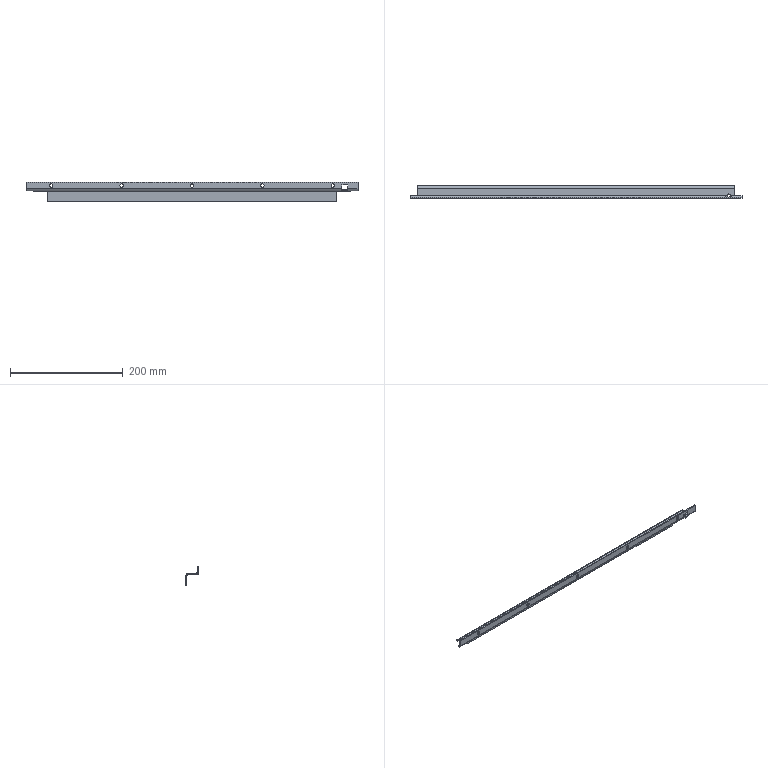Part | NX | features solid 2 | 1 solid | 44 faces | box 590 x 22 x 35 mm | volume 57677 mm3 | plane 26 | cylinder 18 | commonest cylinder face diameters 6 x12 4 x3 8 x3
STEP:
#1=CARTESIAN_POINT('',(1874.5,-1576.5,1027.));
#2=VERTEX_POINT('',#1);
#3=CARTESIAN_POINT('',(1874.5,-1576.5,1025.));
#4=VERTEX_POINT('',#3);
#5=CARTESIAN_POINT('',(1874.5,-1576.5,1616.447));
#6=DIRECTION('',(0.,0.,-1.));
#7=VECTOR('',#6,1000.);
#8=LINE('',#5,#7);
#9=EDGE_CURVE('',#2,#4,#8,.T.);
#10=ORIENTED_EDGE('',*,*,#9,.F.);
#11=CARTESIAN_POINT('',(1874.5,-1570.5,1027.));
#12=VERTEX_POINT('',#11);
#13=CARTESIAN_POINT('',(1874.5,-1573.5,1027.));
#14=DIRECTION('',(0.,0.,1.));
#15=DIRECTION('',(0.,-1.,0.));
#16=AXIS2_PLACEMENT_3D('',#13,#14,#15);
#17=CIRCLE('',#16,3.);
#18=EDGE_CURVE('',#2,#12,#17,.T.);
#19=ORIENTED_EDGE('',*,*,#18,.T.);
#20=CARTESIAN_POINT('',(1874.5,-1570.5,1025.));
#21=VERTEX_POINT('',#20);
#22=CARTESIAN_POINT('',(1874.5,-1570.5,1616.447));
#23=DIRECTION('',(0.,0.,-1.));
#24=VECTOR('',#23,1000.);
#25=LINE('',#22,#24);
#26=EDGE_CURVE('',#21,#12,#25,.F.);
#27=ORIENTED_EDGE('',*,*,#26,.F.);
#28=CARTESIAN_POINT('',(1874.5,-1573.5,1025.));
#29=DIRECTION('',(0.,0.,-1.));
#30=DIRECTION('',(1.,0.,0.));
#31=AXIS2_PLACEMENT_3D('',#28,#29,#30);
#32=CIRCLE('',#31,3.);
#33=EDGE_CURVE('',#21,#4,#32,.T.);
#34=ORIENTED_EDGE('',*,*,#33,.T.);
#35=EDGE_LOOP('',(#10,#19,#27,#34));
#36=FACE_BOUND('',#35,.T.);
#37=CARTESIAN_POINT('',(1874.5,-1573.5,1616.447));
#38=DIRECTION('',(0.,0.,-1.));
#39=DIRECTION('',(0.,1.,0.));
#40=AXIS2_PLACEMENT_3D('',#37,#38,#39);
#41=CYLINDRICAL_SURFACE('',#40,3.);
#42=ADVANCED_FACE('',(#36),#41,.F.);
#43=CARTESIAN_POINT('',(1879.4,-1574.,1025.));
#44=VERTEX_POINT('',#43);
#45=CARTESIAN_POINT('',(1879.5,-1574.,1025.));
#46=VERTEX_POINT('',#45);
#47=CARTESIAN_POINT('',(1879.5,-1574.,1025.));
#48=DIRECTION('',(1.,0.,0.));
#49=VECTOR('',#48,1000.);
#50=LINE('',#47,#49);
#51=EDGE_CURVE('',#44,#46,#50,.T.);
#52=ORIENTED_EDGE('',*,*,#51,.T.);
#53=CARTESIAN_POINT('',(1879.5,-1574.,1027.));
#54=VERTEX_POINT('',#53);
#55=CARTESIAN_POINT('',(1879.5,-1574.,1027.));
#56=DIRECTION('',(0.,0.,-1.));
#57=VECTOR('',#56,1000.);
#58=LINE('',#55,#57);
#59=EDGE_CURVE('',#54,#46,#58,.T.);
#60=ORIENTED_EDGE('',*,*,#59,.F.);
#61=CARTESIAN_POINT('',(1879.4,-1574.,1027.));
#62=VERTEX_POINT('',#61);
#63=CARTESIAN_POINT('',(1879.5,-1574.,1027.));
#64=DIRECTION('',(1.,0.,0.));
#65=VECTOR('',#64,1000.);
#66=LINE('',#63,#65);
#67=EDGE_CURVE('',#62,#54,#66,.T.);
#68=ORIENTED_EDGE('',*,*,#67,.F.);
#69=CARTESIAN_POINT('',(1879.4,-1574.,1027.));
#70=DIRECTION('',(0.,0.,-1.));
#71=VECTOR('',#70,1000.);
#72=LINE('',#69,#71);
#73=EDGE_CURVE('',#62,#44,#72,.T.);
#74=ORIENTED_EDGE('',*,*,#73,.T.);
#75=EDGE_LOOP('',(#52,#60,#68,#74));
#76=FACE_BOUND('',#75,.T.);
#77=CARTESIAN_POINT('',(1879.5,-1574.,1027.));
#78=DIRECTION('',(0.,1.,0.));
#79=DIRECTION('',(0.,0.,-1.));
#80=AXIS2_PLACEMENT_3D('',#77,#78,#79);
#81=PLANE('',#80);
#82=ADVANCED_FACE('',(#76),#81,.F.);
#83=CARTESIAN_POINT('',(1879.4,-1578.,1025.));
#84=VERTEX_POINT('',#83);
#85=CARTESIAN_POINT('',(1879.4,-1578.,1025.));
#86=DIRECTION('',(0.,1.,0.));
#87=VECTOR('',#86,1000.);
#88=LINE('',#85,#87);
#89=EDGE_CURVE('',#84,#44,#88,.T.);
#90=ORIENTED_EDGE('',*,*,#89,.T.);
#91=ORIENTED_EDGE('',*,*,#73,.F.);
#92=CARTESIAN_POINT('',(1879.4,-1578.,1027.));
#93=VERTEX_POINT('',#92);
#94=CARTESIAN_POINT('',(1879.4,-1578.,1027.));
#95=DIRECTION('',(0.,1.,0.));
#96=VECTOR('',#95,1000.);
#97=LINE('',#94,#96);
#98=EDGE_CURVE('',#93,#62,#97,.T.);
#99=ORIENTED_EDGE('',*,*,#98,.F.);
#100=CARTESIAN_POINT('',(1879.4,-1578.,1027.));
#101=DIRECTION('',(0.,0.,-1.));
#102=VECTOR('',#101,1000.);
#103=LINE('',#100,#102);
#104=EDGE_CURVE('',#93,#84,#103,.T.);
#105=ORIENTED_EDGE('',*,*,#104,.T.);
#106=EDGE_LOOP('',(#90,#91,#99,#105));
#107=FACE_BOUND('',#106,.T.);
#108=CARTESIAN_POINT('',(1879.4,-1578.,1027.));
#109=DIRECTION('',(-1.,0.,0.));
#110=DIRECTION('',(0.,0.,1.));
#111=AXIS2_PLACEMENT_3D('',#108,#109,#110);
#112=PLANE('',#111);
#113=ADVANCED_FACE('',(#107),#112,.F.);
#114=CARTESIAN_POINT('',(1869.6,-1578.,1025.));
#115=VERTEX_POINT('',#114);
#116=CARTESIAN_POINT('',(1879.4,-1578.,1025.));
#117=DIRECTION('',(1.,0.,0.));
#118=VECTOR('',#117,1000.);
#119=LINE('',#116,#118);
#120=EDGE_CURVE('',#115,#84,#119,.T.);
#121=ORIENTED_EDGE('',*,*,#120,.T.);
#122=ORIENTED_EDGE('',*,*,#104,.F.);
#123=CARTESIAN_POINT('',(1869.6,-1578.,1027.));
#124=VERTEX_POINT('',#123);
#125=CARTESIAN_POINT('',(1879.4,-1578.,1027.));
#126=DIRECTION('',(1.,0.,0.));
#127=VECTOR('',#126,1000.);
#128=LINE('',#125,#127);
#129=EDGE_CURVE('',#124,#93,#128,.T.);
#130=ORIENTED_EDGE('',*,*,#129,.F.);
#131=CARTESIAN_POINT('',(1869.6,-1578.,1027.));
#132=DIRECTION('',(0.,0.,-1.));
#133=VECTOR('',#132,1000.);
#134=LINE('',#131,#133);
#135=EDGE_CURVE('',#124,#115,#134,.T.);
#136=ORIENTED_EDGE('',*,*,#135,.T.);
#137=EDGE_LOOP('',(#121,#122,#130,#136));
#138=FACE_BOUND('',#137,.T.);
#139=CARTESIAN_POINT('',(1879.4,-1578.,1027.));
#140=DIRECTION('',(0.,1.,0.));
#141=DIRECTION('',(0.,0.,-1.));
#142=AXIS2_PLACEMENT_3D('',#139,#140,#141);
#143=PLANE('',#142);
#144=ADVANCED_FACE('',(#138),#143,.F.);
#145=CARTESIAN_POINT('',(1869.6,-1574.,1025.));
#146=VERTEX_POINT('',#145);
#147=CARTESIAN_POINT('',(1869.6,-1574.,1025.));
#148=DIRECTION('',(0.,-1.,0.));
#149=VECTOR('',#148,1000.);
#150=LINE('',#147,#149);
#151=EDGE_CURVE('',#146,#115,#150,.T.);
#152=ORIENTED_EDGE('',*,*,#151,.T.);
#153=ORIENTED_EDGE('',*,*,#135,.F.);
#154=CARTESIAN_POINT('',(1869.6,-1574.,1027.));
#155=VERTEX_POINT('',#154);
#156=CARTESIAN_POINT('',(1869.6,-1574.,1027.));
#157=DIRECTION('',(0.,-1.,0.));
#158=VECTOR('',#157,1000.);
#159=LINE('',#156,#158);
#160=EDGE_CURVE('',#155,#124,#159,.T.);
#161=ORIENTED_EDGE('',*,*,#160,.F.);
#162=CARTESIAN_POINT('',(1869.6,-1574.,1027.));
#163=DIRECTION('',(0.,0.,-1.));
#164=VECTOR('',#163,1000.);
#165=LINE('',#162,#164);
#166=EDGE_CURVE('',#155,#146,#165,.T.);
#167=ORIENTED_EDGE('',*,*,#166,.T.);
#168=EDGE_LOOP('',(#152,#153,#161,#167));
#169=FACE_BOUND('',#168,.T.);
#170=CARTESIAN_POINT('',(1869.6,-1574.,1027.));
#171=DIRECTION('',(1.,0.,0.));
#172=DIRECTION('',(0.,0.,1.));
#173=AXIS2_PLACEMENT_3D('',#170,#171,#172);
#174=PLANE('',#173);
#175=ADVANCED_FACE('',(#169),#174,.F.);
#176=CARTESIAN_POINT('',(1869.5,-1574.,1025.));
#177=VERTEX_POINT('',#176);
#178=CARTESIAN_POINT('',(1869.6,-1574.,1025.));
#179=DIRECTION('',(1.,0.,0.));
#180=VECTOR('',#179,1000.);
#181=LINE('',#178,#180);
#182=EDGE_CURVE('',#177,#146,#181,.T.);
#183=ORIENTED_EDGE('',*,*,#182,.T.);
#184=ORIENTED_EDGE('',*,*,#166,.F.);
#185=CARTESIAN_POINT('',(1869.5,-1574.,1027.));
#186=VERTEX_POINT('',#185);
#187=CARTESIAN_POINT('',(1869.6,-1574.,1027.));
#188=DIRECTION('',(1.,0.,0.));
#189=VECTOR('',#188,1000.);
#190=LINE('',#187,#189);
#191=EDGE_CURVE('',#186,#155,#190,.T.);
#192=ORIENTED_EDGE('',*,*,#191,.F.);
#193=CARTESIAN_POINT('',(1869.5,-1574.,1027.));
#194=DIRECTION('',(0.,0.,-1.));
#195=VECTOR('',#194,1000.);
#196=LINE('',#193,#195);
#197=EDGE_CURVE('',#186,#177,#196,.T.);
#198=ORIENTED_EDGE('',*,*,#197,.T.);
#199=EDGE_LOOP('',(#183,#184,#192,#198));
#200=FACE_BOUND('',#199,.T.);
#201=CARTESIAN_POINT('',(1869.6,-1574.,1027.));
#202=DIRECTION('',(0.,1.,0.));
#203=DIRECTION('',(0.,0.,-1.));
#204=AXIS2_PLACEMENT_3D('',#201,#202,#203);
#205=PLANE('',#204);
#206=ADVANCED_FACE('',(#200),#205,.F.);
#207=CARTESIAN_POINT('',(1869.5,-1576.,1035.));
#208=VERTEX_POINT('',#207);
#209=CARTESIAN_POINT('',(1869.5,-1578.,1035.));
#210=VERTEX_POINT('',#209);
#211=CARTESIAN_POINT('',(1869.5,-1578.,1035.));
#212=DIRECTION('',(0.,-1.,0.));
#213=VECTOR('',#212,1000.);
#214=LINE('',#211,#213);
#215=EDGE_CURVE('',#208,#210,#214,.T.);
#216=ORIENTED_EDGE('',*,*,#215,.F.);
#217=CARTESIAN_POINT('',(1879.5,-1576.,1035.));
#218=VERTEX_POINT('',#217);
#219=CARTESIAN_POINT('',(1898.,-1576.,1035.));
#220=DIRECTION('',(-1.,0.,0.));
#221=VECTOR('',#220,1000.);
#222=LINE('',#219,#221);
#223=EDGE_CURVE('',#218,#208,#222,.T.);
#224=ORIENTED_EDGE('',*,*,#223,.F.);
#225=CARTESIAN_POINT('',(1879.5,-1578.,1035.));
#226=VERTEX_POINT('',#225);
#227=CARTESIAN_POINT('',(1879.5,-1578.,1035.));
#228=DIRECTION('',(0.,-1.,0.));
#229=VECTOR('',#228,1000.);
#230=LINE('',#227,#229);
#231=EDGE_CURVE('',#218,#226,#230,.T.);
#232=ORIENTED_EDGE('',*,*,#231,.T.);
#233=CARTESIAN_POINT('',(1898.,-1578.,1035.));
#234=DIRECTION('',(-1.,0.,0.));
#235=VECTOR('',#234,1000.);
#236=LINE('',#233,#235);
#237=EDGE_CURVE('',#226,#210,#236,.T.);
#238=ORIENTED_EDGE('',*,*,#237,.T.);
#239=EDGE_LOOP('',(#216,#224,#232,#238));
#240=FACE_BOUND('',#239,.T.);
#241=CARTESIAN_POINT('',(1898.,-1578.,1035.));
#242=DIRECTION('',(0.,0.,-1.));
#243=DIRECTION('',(0.,-1.,0.));
#244=AXIS2_PLACEMENT_3D('',#241,#242,#243);
#245=PLANE('',#244);
#246=ADVANCED_FACE('',(#240),#245,.T.);
#247=CARTESIAN_POINT('',(1885.,-1558.,1023.));
#248=VERTEX_POINT('',#247);
#249=CARTESIAN_POINT('',(1885.,-1560.,1025.));
#250=VERTEX_POINT('',#249);
#251=CARTESIAN_POINT('',(1885.,-1560.,1023.));
#252=DIRECTION('',(1.,0.,0.));
#253=DIRECTION('',(0.,0.,-1.));
#254=AXIS2_PLACEMENT_3D('',#251,#252,#253);
#255=CIRCLE('',#254,2.);
#256=EDGE_CURVE('',#248,#250,#255,.T.);
#257=ORIENTED_EDGE('',*,*,#256,.F.);
#258=CARTESIAN_POINT('',(1885.,-1556.,1023.));
#259=VERTEX_POINT('',#258);
#260=CARTESIAN_POINT('',(1885.,-1558.,1023.));
#261=DIRECTION('',(0.,-1.,0.));
#262=VECTOR('',#261,1000.);
#263=LINE('',#260,#262);
#264=EDGE_CURVE('',#259,#248,#263,.T.);
#265=ORIENTED_EDGE('',*,*,#264,.F.);
#266=CARTESIAN_POINT('',(1885.,-1560.,1027.));
#267=VERTEX_POINT('',#266);
#268=CARTESIAN_POINT('',(1885.,-1560.,1023.));
#269=DIRECTION('',(1.,0.,0.));
#270=DIRECTION('',(0.,0.,-1.));
#271=AXIS2_PLACEMENT_3D('',#268,#269,#270);
#272=CIRCLE('',#271,4.);
#273=EDGE_CURVE('',#259,#267,#272,.T.);
#274=ORIENTED_EDGE('',*,*,#273,.T.);
#275=CARTESIAN_POINT('',(1885.,-1574.,1027.));
#276=VERTEX_POINT('',#275);
#277=CARTESIAN_POINT('',(1885.,-1578.,1027.));
#278=DIRECTION('',(0.,-1.,0.));
#279=VECTOR('',#278,1000.);
#280=LINE('',#277,#279);
#281=EDGE_CURVE('',#267,#276,#280,.T.);
#282=ORIENTED_EDGE('',*,*,#281,.T.);
#283=CARTESIAN_POINT('',(1885.,-1574.,1025.));
#284=VERTEX_POINT('',#283);
#285=CARTESIAN_POINT('',(1885.,-1574.,1025.));
#286=DIRECTION('',(0.,0.,-1.));
#287=VECTOR('',#286,1000.);
#288=LINE('',#285,#287);
#289=EDGE_CURVE('',#276,#284,#288,.T.);
#290=ORIENTED_EDGE('',*,*,#289,.T.);
#291=CARTESIAN_POINT('',(1885.,-1578.,1025.));
#292=DIRECTION('',(0.,-1.,0.));
#293=VECTOR('',#292,1000.);
#294=LINE('',#291,#293);
#295=EDGE_CURVE('',#250,#284,#294,.T.);
#296=ORIENTED_EDGE('',*,*,#295,.F.);
#297=EDGE_LOOP('',(#257,#265,#274,#282,#290,#296));
#298=FACE_BOUND('',#297,.T.);
#299=CARTESIAN_POINT('',(1885.,-1560.,1023.));
#300=DIRECTION('',(1.,0.,0.));
#301=DIRECTION('',(0.,0.,1.));
#302=AXIS2_PLACEMENT_3D('',#299,#300,#301);
#303=PLANE('',#302);
#304=ADVANCED_FACE('',(#298),#303,.T.);
#305=CARTESIAN_POINT('',(1898.,-1574.,1027.));
#306=VERTEX_POINT('',#305);
#307=CARTESIAN_POINT('',(1898.,-1574.,1025.));
#308=VERTEX_POINT('',#307);
#309=CARTESIAN_POINT('',(1898.,-1574.,1025.));
#310=DIRECTION('',(0.,0.,-1.));
#311=VECTOR('',#310,1000.);
#312=LINE('',#309,#311);
#313=EDGE_CURVE('',#306,#308,#312,.T.);
#314=ORIENTED_EDGE('',*,*,#313,.T.);
#315=CARTESIAN_POINT('',(1898.,-1574.,1025.));
#316=DIRECTION('',(-1.,0.,0.));
#317=VECTOR('',#316,1000.);
#318=LINE('',#315,#317);
#319=EDGE_CURVE('',#308,#284,#318,.T.);
#320=ORIENTED_EDGE('',*,*,#319,.T.);
#321=ORIENTED_EDGE('',*,*,#289,.F.);
#322=CARTESIAN_POINT('',(1898.,-1574.,1027.));
#323=DIRECTION('',(-1.,0.,0.));
#324=VECTOR('',#323,1000.);
#325=LINE('',#322,#324);
#326=EDGE_CURVE('',#306,#276,#325,.T.);
#327=ORIENTED_EDGE('',*,*,#326,.F.);
#328=EDGE_LOOP('',(#314,#320,#321,#327));
#329=FACE_BOUND('',#328,.T.);
#330=CARTESIAN_POINT('',(1898.,-1574.,1025.));
#331=DIRECTION('',(0.,1.,0.));
#332=DIRECTION('',(0.,0.,-1.));
#333=AXIS2_PLACEMENT_3D('',#330,#331,#332);
#334=PLANE('',#333);
#335=ADVANCED_FACE('',(#329),#334,.T.);
#336=CARTESIAN_POINT('',(1321.,-1574.,1027.));
#337=VERTEX_POINT('',#336);
#338=CARTESIAN_POINT('',(1321.,-1560.,1027.));
#339=VERTEX_POINT('',#338);
#340=CARTESIAN_POINT('',(1321.,-1578.,1027.));
#341=DIRECTION('',(0.,1.,0.));
#342=VECTOR('',#341,1000.);
#343=LINE('',#340,#342);
#344=EDGE_CURVE('',#337,#339,#343,.T.);
#345=ORIENTED_EDGE('',*,*,#344,.T.);
#346=CARTESIAN_POINT('',(1321.,-1556.,1023.));
#347=VERTEX_POINT('',#346);
#348=CARTESIAN_POINT('',(1321.,-1560.,1023.));
#349=DIRECTION('',(-1.,0.,0.));
#350=DIRECTION('',(0.,0.,-1.));
#351=AXIS2_PLACEMENT_3D('',#348,#349,#350);
#352=CIRCLE('',#351,4.);
#353=EDGE_CURVE('',#339,#347,#352,.T.);
#354=ORIENTED_EDGE('',*,*,#353,.T.);
#355=CARTESIAN_POINT('',(1321.,-1558.,1023.));
#356=VERTEX_POINT('',#355);
#357=CARTESIAN_POINT('',(1321.,-1558.,1023.));
#358=DIRECTION('',(0.,-1.,0.));
#359=VECTOR('',#358,1000.);
#360=LINE('',#357,#359);
#361=EDGE_CURVE('',#347,#356,#360,.T.);
#362=ORIENTED_EDGE('',*,*,#361,.T.);
#363=CARTESIAN_POINT('',(1321.,-1560.,1025.));
#364=VERTEX_POINT('',#363);
#365=CARTESIAN_POINT('',(1321.,-1560.,1023.));
#366=DIRECTION('',(-1.,0.,0.));
#367=DIRECTION('',(0.,0.,1.));
#368=AXIS2_PLACEMENT_3D('',#365,#366,#367);
#369=CIRCLE('',#368,2.);
#370=EDGE_CURVE('',#364,#356,#369,.T.);
#371=ORIENTED_EDGE('',*,*,#370,.F.);
#372=CARTESIAN_POINT('',(1321.,-1574.,1025.));
#373=VERTEX_POINT('',#372);
#374=CARTESIAN_POINT('',(1321.,-1578.,1025.));
#375=DIRECTION('',(0.,1.,0.));
#376=VECTOR('',#375,1000.);
#377=LINE('',#374,#376);
#378=EDGE_CURVE('',#373,#364,#377,.T.);
#379=ORIENTED_EDGE('',*,*,#378,.F.);
#380=CARTESIAN_POINT('',(1321.,-1574.,1025.));
#381=DIRECTION('',(0.,0.,-1.));
#382=VECTOR('',#381,1000.);
#383=LINE('',#380,#382);
#384=EDGE_CURVE('',#337,#373,#383,.T.);
#385=ORIENTED_EDGE('',*,*,#384,.F.);
#386=EDGE_LOOP('',(#345,#354,#362,#371,#379,#385));
#387=FACE_BOUND('',#386,.T.);
#388=CARTESIAN_POINT('',(1321.,-1578.,1025.));
#389=DIRECTION('',(1.,0.,0.));
#390=DIRECTION('',(0.,0.,1.));
#391=AXIS2_PLACEMENT_3D('',#388,#389,#390);
#392=PLANE('',#391);
#393=ADVANCED_FACE('',(#387),#392,.F.);
#394=ORIENTED_EDGE('',*,*,#384,.T.);
#395=CARTESIAN_POINT('',(1308.,-1574.,1025.));
#396=VERTEX_POINT('',#395);
#397=CARTESIAN_POINT('',(1898.,-1574.,1025.));
#398=DIRECTION('',(-1.,0.,0.));
#399=VECTOR('',#398,1000.);
#400=LINE('',#397,#399);
#401=EDGE_CURVE('',#373,#396,#400,.T.);
#402=ORIENTED_EDGE('',*,*,#401,.T.);
#403=CARTESIAN_POINT('',(1308.,-1574.,1027.));
#404=VERTEX_POINT('',#403);
#405=CARTESIAN_POINT('',(1308.,-1574.,1025.));
#406=DIRECTION('',(0.,0.,-1.));
#407=VECTOR('',#406,1000.);
#408=LINE('',#405,#407);
#409=EDGE_CURVE('',#404,#396,#408,.T.);
#410=ORIENTED_EDGE('',*,*,#409,.F.);
#411=CARTESIAN_POINT('',(1898.,-1574.,1027.));
#412=DIRECTION('',(-1.,0.,0.));
#413=VECTOR('',#412,1000.);
#414=LINE('',#411,#413);
#415=EDGE_CURVE('',#337,#404,#414,.T.);
#416=ORIENTED_EDGE('',*,*,#415,.F.);
#417=EDGE_LOOP('',(#394,#402,#410,#416));
#418=FACE_BOUND('',#417,.T.);
#419=CARTESIAN_POINT('',(1898.,-1574.,1025.));
#420=DIRECTION('',(0.,1.,0.));
#421=DIRECTION('',(0.,0.,-1.));
#422=AXIS2_PLACEMENT_3D('',#419,#420,#421);
#423=PLANE('',#422);
#424=ADVANCED_FACE('',(#418),#423,.T.);
#425=CARTESIAN_POINT('',(1603.,-1578.,1031.));
#426=VERTEX_POINT('',#425);
#427=CARTESIAN_POINT('',(1603.,-1576.,1031.));
#428=VERTEX_POINT('',#427);
#429=CARTESIAN_POINT('',(1603.,-2167.447,1031.));
#430=DIRECTION('',(0.,1.,0.));
#431=VECTOR('',#430,1000.);
#432=LINE('',#429,#431);
#433=EDGE_CURVE('',#426,#428,#432,.T.);
#434=ORIENTED_EDGE('',*,*,#433,.F.);
#435=CARTESIAN_POINT('',(1603.,-1578.,1037.));
#436=VERTEX_POINT('',#435);
#437=CARTESIAN_POINT('',(1603.,-1578.,1034.));
#438=DIRECTION('',(0.,1.,0.));
#439=DIRECTION('',(0.,0.,1.));
#440=AXIS2_PLACEMENT_3D('',#437,#438,#439);
#441=CIRCLE('',#440,3.);
#442=EDGE_CURVE('',#436,#426,#441,.T.);
#443=ORIENTED_EDGE('',*,*,#442,.F.);
#444=CARTESIAN_POINT('',(1603.,-1576.,1037.));
#445=VERTEX_POINT('',#444);
#446=CARTESIAN_POINT('',(1603.,-2167.447,1037.));
#447=DIRECTION('',(0.,1.,0.));
#448=VECTOR('',#447,1000.);
#449=LINE('',#446,#448);
#450=EDGE_CURVE('',#445,#436,#449,.F.);
#451=ORIENTED_EDGE('',*,*,#450,.F.);
#452=CARTESIAN_POINT('',(1603.,-1576.,1034.));
#453=DIRECTION('',(0.,1.,0.));
#454=DIRECTION('',(-1.,0.,0.));
#455=AXIS2_PLACEMENT_3D('',#452,#453,#454);
#456=CIRCLE('',#455,3.);
#457=EDGE_CURVE('',#445,#428,#456,.T.);
#458=ORIENTED_EDGE('',*,*,#457,.T.);
#459=EDGE_LOOP('',(#434,#443,#451,#458));
#460=FACE_BOUND('',#459,.T.);
#461=CARTESIAN_POINT('',(1603.,-2167.447,1034.));
#462=DIRECTION('',(0.,1.,0.));
#463=DIRECTION('',(0.,0.,1.));
#464=AXIS2_PLACEMENT_3D('',#461,#462,#463);
#465=CYLINDRICAL_SURFACE('',#464,3.);
#466=ADVANCED_FACE('',(#460),#465,.F.);
#467=CARTESIAN_POINT('',(1853.,-1578.,1031.));
#468=VERTEX_POINT('',#467);
#469=CARTESIAN_POINT('',(1853.,-1576.,1031.));
#470=VERTEX_POINT('',#469);
#471=CARTESIAN_POINT('',(1853.,-2167.447,1031.));
#472=DIRECTION('',(0.,1.,0.));
#473=VECTOR('',#472,1000.);
#474=LINE('',#471,#473);
#475=EDGE_CURVE('',#468,#470,#474,.T.);
#476=ORIENTED_EDGE('',*,*,#475,.F.);
#477=CARTESIAN_POINT('',(1853.,-1578.,1037.));
#478=VERTEX_POINT('',#477);
#479=CARTESIAN_POINT('',(1853.,-1578.,1034.));
#480=DIRECTION('',(0.,1.,0.));
#481=DIRECTION('',(0.,0.,1.));
#482=AXIS2_PLACEMENT_3D('',#479,#480,#481);
#483=CIRCLE('',#482,3.);
#484=EDGE_CURVE('',#478,#468,#483,.T.);
#485=ORIENTED_EDGE('',*,*,#484,.F.);
#486=CARTESIAN_POINT('',(1853.,-1576.,1037.));
#487=VERTEX_POINT('',#486);
#488=CARTESIAN_POINT('',(1853.,-2167.447,1037.));
#489=DIRECTION('',(0.,1.,0.));
#490=VECTOR('',#489,1000.);
#491=LINE('',#488,#490);
#492=EDGE_CURVE('',#487,#478,#491,.F.);
#493=ORIENTED_EDGE('',*,*,#492,.F.);
#494=CARTESIAN_POINT('',(1853.,-1576.,1034.));
#495=DIRECTION('',(0.,1.,0.));
#496=DIRECTION('',(-1.,0.,0.));
#497=AXIS2_PLACEMENT_3D('',#494,#495,#496);
#498=CIRCLE('',#497,3.);
#499=EDGE_CURVE('',#487,#470,#498,.T.);
#500=ORIENTED_EDGE('',*,*,#499,.T.);
#501=EDGE_LOOP('',(#476,#485,#493,#500));
#502=FACE_BOUND('',#501,.T.);
#503=CARTESIAN_POINT('',(1853.,-2167.447,1034.));
#504=DIRECTION('',(0.,1.,0.));
#505=DIRECTION('',(0.,0.,1.));
#506=AXIS2_PLACEMENT_3D('',#503,#504,#505);
#507=CYLINDRICAL_SURFACE('',#506,3.);
#508=ADVANCED_FACE('',(#502),#507,.F.);
#509=CARTESIAN_POINT('',(1728.,-1578.,1031.));
#510=VERTEX_POINT('',#509);
#511=CARTESIAN_POINT('',(1728.,-1576.,1031.));
#512=VERTEX_POINT('',#511);
#513=CARTESIAN_POINT('',(1728.,-2167.447,1031.));
#514=DIRECTION('',(0.,1.,0.));
#515=VECTOR('',#514,1000.);
#516=LINE('',#513,#515);
#517=EDGE_CURVE('',#510,#512,#516,.T.);
#518=ORIENTED_EDGE('',*,*,#517,.F.);
#519=CARTESIAN_POINT('',(1728.,-1578.,1037.));
#520=VERTEX_POINT('',#519);
#521=CARTESIAN_POINT('',(1728.,-1578.,1034.));
#522=DIRECTION('',(0.,1.,0.));
#523=DIRECTION('',(0.,0.,1.));
#524=AXIS2_PLACEMENT_3D('',#521,#522,#523);
#525=CIRCLE('',#524,3.);
#526=EDGE_CURVE('',#520,#510,#525,.T.);
#527=ORIENTED_EDGE('',*,*,#526,.F.);
#528=CARTESIAN_POINT('',(1728.,-1576.,1037.));
#529=VERTEX_POINT('',#528);
#530=CARTESIAN_POINT('',(1728.,-2167.447,1037.));
#531=DIRECTION('',(0.,1.,0.));
#532=VECTOR('',#531,1000.);
#533=LINE('',#530,#532);
#534=EDGE_CURVE('',#529,#520,#533,.F.);
#535=ORIENTED_EDGE('',*,*,#534,.F.);
#536=CARTESIAN_POINT('',(1728.,-1576.,1034.));
#537=DIRECTION('',(0.,1.,0.));
#538=DIRECTION('',(-1.,0.,0.));
#539=AXIS2_PLACEMENT_3D('',#536,#537,#538);
#540=CIRCLE('',#539,3.);
#541=EDGE_CURVE('',#529,#512,#540,.T.);
#542=ORIENTED_EDGE('',*,*,#541,.T.);
#543=EDGE_LOOP('',(#518,#527,#535,#542));
#544=FACE_BOUND('',#543,.T.);
#545=CARTESIAN_POINT('',(1728.,-2167.447,1034.));
#546=DIRECTION('',(0.,1.,0.));
#547=DIRECTION('',(0.,0.,1.));
#548=AXIS2_PLACEMENT_3D('',#545,#546,#547);
#549=CYLINDRICAL_SURFACE('',#548,3.);
#550=ADVANCED_FACE('',(#544),#549,.F.);
#551=CARTESIAN_POINT('',(1353.,-1578.,1031.));
#552=VERTEX_POINT('',#551);
#553=CARTESIAN_POINT('',(1353.,-1576.,1031.));
#554=VERTEX_POINT('',#553);
#555=CARTESIAN_POINT('',(1353.,-2167.447,1031.));
#556=DIRECTION('',(0.,1.,0.));
#557=VECTOR('',#556,1000.);
#558=LINE('',#555,#557);
#559=EDGE_CURVE('',#552,#554,#558,.T.);
#560=ORIENTED_EDGE('',*,*,#559,.F.);
#561=CARTESIAN_POINT('',(1353.,-1578.,1037.));
#562=VERTEX_POINT('',#561);
#563=CARTESIAN_POINT('',(1353.,-1578.,1034.));
#564=DIRECTION('',(0.,1.,0.));
#565=DIRECTION('',(0.,0.,1.));
#566=AXIS2_PLACEMENT_3D('',#563,#564,#565);
#567=CIRCLE('',#566,3.);
#568=EDGE_CURVE('',#562,#552,#567,.T.);
#569=ORIENTED_EDGE('',*,*,#568,.F.);
#570=CARTESIAN_POINT('',(1353.,-1576.,1037.));
#571=VERTEX_POINT('',#570);
#572=CARTESIAN_POINT('',(1353.,-2167.447,1037.));
#573=DIRECTION('',(0.,1.,0.));
#574=VECTOR('',#573,1000.);
#575=LINE('',#572,#574);
#576=EDGE_CURVE('',#571,#562,#575,.F.);
#577=ORIENTED_EDGE('',*,*,#576,.F.);
#578=CARTESIAN_POINT('',(1353.,-1576.,1034.));
#579=DIRECTION('',(0.,1.,0.));
#580=DIRECTION('',(-1.,0.,0.));
#581=AXIS2_PLACEMENT_3D('',#578,#579,#580);
#582=CIRCLE('',#581,3.);
#583=EDGE_CURVE('',#571,#554,#582,.T.);
#584=ORIENTED_EDGE('',*,*,#583,.T.);
#585=EDGE_LOOP('',(#560,#569,#577,#584));
#586=FACE_BOUND('',#585,.T.);
#587=CARTESIAN_POINT('',(1353.,-2167.447,1034.));
#588=DIRECTION('',(0.,1.,0.));
#589=DIRECTION('',(0.,0.,1.));
#590=AXIS2_PLACEMENT_3D('',#587,#588,#589);
#591=CYLINDRICAL_SURFACE('',#590,3.);
#592=ADVANCED_FACE('',(#586),#591,.F.);
#593=CARTESIAN_POINT('',(1478.,-1578.,1031.));
#594=VERTEX_POINT('',#593);
#595=CARTESIAN_POINT('',(1478.,-1576.,1031.));
#596=VERTEX_POINT('',#595);
#597=CARTESIAN_POINT('',(1478.,-2167.447,1031.));
#598=DIRECTION('',(0.,1.,0.));
#599=VECTOR('',#598,1000.);
#600=LINE('',#597,#599);
#601=EDGE_CURVE('',#594,#596,#600,.T.);
#602=ORIENTED_EDGE('',*,*,#601,.F.);
#603=CARTESIAN_POINT('',(1478.,-1578.,1037.));
#604=VERTEX_POINT('',#603);
#605=CARTESIAN_POINT('',(1478.,-1578.,1034.));
#606=DIRECTION('',(0.,1.,0.));
#607=DIRECTION('',(0.,0.,1.));
#608=AXIS2_PLACEMENT_3D('',#605,#606,#607);
#609=CIRCLE('',#608,3.);
#610=EDGE_CURVE('',#604,#594,#609,.T.);
#611=ORIENTED_EDGE('',*,*,#610,.F.);
#612=CARTESIAN_POINT('',(1478.,-1576.,1037.));
#613=VERTEX_POINT('',#612);
#614=CARTESIAN_POINT('',(1478.,-2167.447,1037.));
#615=DIRECTION('',(0.,1.,0.));
#616=VECTOR('',#615,1000.);
#617=LINE('',#614,#616);
#618=EDGE_CURVE('',#613,#604,#617,.F.);
#619=ORIENTED_EDGE('',*,*,#618,.F.);
#620=CARTESIAN_POINT('',(1478.,-1576.,1034.));
#621=DIRECTION('',(0.,1.,0.));
#622=DIRECTION('',(-1.,0.,0.));
#623=AXIS2_PLACEMENT_3D('',#620,#621,#622);
#624=CIRCLE('',#623,3.);
#625=EDGE_CURVE('',#613,#596,#624,.T.);
#626=ORIENTED_EDGE('',*,*,#625,.T.);
#627=EDGE_LOOP('',(#602,#611,#619,#626));
#628=FACE_BOUND('',#627,.T.);
#629=CARTESIAN_POINT('',(1478.,-2167.447,1034.));
#630=DIRECTION('',(0.,1.,0.));
#631=DIRECTION('',(0.,0.,1.));
#632=AXIS2_PLACEMENT_3D('',#629,#630,#631);
#633=CYLINDRICAL_SURFACE('',#632,3.);
#634=ADVANCED_FACE('',(#628),#633,.F.);
#635=CARTESIAN_POINT('',(1860.,-1556.,1023.));
#636=VERTEX_POINT('',#635);
#637=CARTESIAN_POINT('',(1860.,-1558.,1023.));
#638=VERTEX_POINT('',#637);
#639=CARTESIAN_POINT('',(1860.,-1558.,1023.));
#640=DIRECTION('',(0.,-1.,0.));
#641=VECTOR('',#640,1000.);
#642=LINE('',#639,#641);
#643=EDGE_CURVE('',#636,#638,#642,.T.);
#644=ORIENTED_EDGE('',*,*,#643,.T.);
#645=CARTESIAN_POINT('',(1860.,-1558.,1005.));
#646=VERTEX_POINT('',#645);
#647=CARTESIAN_POINT('',(1860.,-1558.,1025.));
#648=DIRECTION('',(0.,0.,1.));
#649=VECTOR('',#648,1000.);
#650=LINE('',#647,#649);
#651=EDGE_CURVE('',#646,#638,#650,.T.);
#652=ORIENTED_EDGE('',*,*,#651,.F.);
#653=CARTESIAN_POINT('',(1860.,-1556.,1005.));
#654=VERTEX_POINT('',#653);
#655=CARTESIAN_POINT('',(1860.,-1558.,1005.));
#656=DIRECTION('',(0.,-1.,0.));
#657=VECTOR('',#656,1000.);
#658=LINE('',#655,#657);
#659=EDGE_CURVE('',#654,#646,#658,.T.);
#660=ORIENTED_EDGE('',*,*,#659,.F.);
#661=CARTESIAN_POINT('',(1860.,-1556.,1025.));
#662=DIRECTION('',(0.,0.,1.));
#663=VECTOR('',#662,1000.);
#664=LINE('',#661,#663);
#665=EDGE_CURVE('',#654,#636,#664,.T.);
#666=ORIENTED_EDGE('',*,*,#665,.T.);
#667=EDGE_LOOP('',(#644,#652,#660,#666));
#668=FACE_BOUND('',#667,.T.);
#669=CARTESIAN_POINT('',(1860.,-1558.,1025.));
#670=DIRECTION('',(-1.,0.,0.));
#671=DIRECTION('',(0.,0.,1.));
#672=AXIS2_PLACEMENT_3D('',#669,#670,#671);
#673=PLANE('',#672);
#674=ADVANCED_FACE('',(#668),#673,.F.);
#675=CARTESIAN_POINT('',(1898.,-1556.,1023.));
#676=DIRECTION('',(-1.,0.,0.));
#677=VECTOR('',#676,1000.);
#678=LINE('',#675,#677);
#679=EDGE_CURVE('',#259,#636,#678,.T.);
#680=ORIENTED_EDGE('',*,*,#679,.F.);
#681=ORIENTED_EDGE('',*,*,#264,.T.);
#682=CARTESIAN_POINT('',(1898.,-1558.,1023.));
#683=DIRECTION('',(-1.,0.,0.));
#684=VECTOR('',#683,1000.);
#685=LINE('',#682,#684);
#686=EDGE_CURVE('',#248,#638,#685,.T.);
#687=ORIENTED_EDGE('',*,*,#686,.T.);
#688=ORIENTED_EDGE('',*,*,#643,.F.);
#689=EDGE_LOOP('',(#680,#681,#687,#688));
#690=FACE_BOUND('',#689,.T.);
#691=CARTESIAN_POINT('',(1898.,-1558.,1023.));
#692=DIRECTION('',(0.,0.,-1.));
#693=DIRECTION('',(0.,-1.,0.));
#694=AXIS2_PLACEMENT_3D('',#691,#692,#693);
#695=PLANE('',#694);
#696=ADVANCED_FACE('',(#690),#695,.T.);
#697=CARTESIAN_POINT('',(1346.,-1556.,1005.));
#698=VERTEX_POINT('',#697);
#699=CARTESIAN_POINT('',(1346.,-1556.,1023.));
#700=VERTEX_POINT('',#699);
#701=CARTESIAN_POINT('',(1346.,-1556.,1025.));
#702=DIRECTION('',(0.,0.,1.));
#703=VECTOR('',#702,1000.);
#704=LINE('',#701,#703);
#705=EDGE_CURVE('',#698,#700,#704,.T.);
#706=ORIENTED_EDGE('',*,*,#705,.F.);
#707=CARTESIAN_POINT('',(1346.,-1558.,1005.));
#708=VERTEX_POINT('',#707);
#709=CARTESIAN_POINT('',(1346.,-1558.,1005.));
#710=DIRECTION('',(0.,-1.,0.));
#711=VECTOR('',#710,1000.);
#712=LINE('',#709,#711);
#713=EDGE_CURVE('',#698,#708,#712,.T.);
#714=ORIENTED_EDGE('',*,*,#713,.T.);
#715=CARTESIAN_POINT('',(1346.,-1558.,1023.));
#716=VERTEX_POINT('',#715);
#717=CARTESIAN_POINT('',(1346.,-1558.,1025.));
#718=DIRECTION('',(0.,0.,1.));
#719=VECTOR('',#718,1000.);
#720=LINE('',#717,#719);
#721=EDGE_CURVE('',#708,#716,#720,.T.);
#722=ORIENTED_EDGE('',*,*,#721,.T.);
#723=CARTESIAN_POINT('',(1346.,-1558.,1023.));
#724=DIRECTION('',(0.,-1.,0.));
#725=VECTOR('',#724,1000.);
#726=LINE('',#723,#725);
#727=EDGE_CURVE('',#700,#716,#726,.T.);
#728=ORIENTED_EDGE('',*,*,#727,.F.);
#729=EDGE_LOOP('',(#706,#714,#722,#728));
#730=FACE_BOUND('',#729,.T.);
#731=CARTESIAN_POINT('',(1346.,-1558.,1025.));
#732=DIRECTION('',(-1.,0.,0.));
#733=DIRECTION('',(0.,0.,1.));
#734=AXIS2_PLACEMENT_3D('',#731,#732,#733);
#735=PLANE('',#734);
#736=ADVANCED_FACE('',(#730),#735,.T.);
#737=CARTESIAN_POINT('',(1898.,-1558.,1005.));
#738=DIRECTION('',(-1.,0.,0.));
#739=VECTOR('',#738,1000.);
#740=LINE('',#737,#739);
#741=EDGE_CURVE('',#646,#708,#740,.T.);
#742=ORIENTED_EDGE('',*,*,#741,.F.);
#743=ORIENTED_EDGE('',*,*,#651,.T.);
#744=CARTESIAN_POINT('',(1898.,-1558.,1023.));
#745=DIRECTION('',(-1.,0.,0.));
#746=VECTOR('',#745,1000.);
#747=LINE('',#744,#746);
#748=EDGE_CURVE('',#638,#716,#747,.T.);
#749=ORIENTED_EDGE('',*,*,#748,.T.);
#750=ORIENTED_EDGE('',*,*,#721,.F.);
#751=EDGE_LOOP('',(#742,#743,#749,#750));
#752=FACE_BOUND('',#751,.T.);
#753=CARTESIAN_POINT('',(1898.,-1558.,1025.));
#754=DIRECTION('',(0.,1.,0.));
#755=DIRECTION('',(0.,0.,-1.));
#756=AXIS2_PLACEMENT_3D('',#753,#754,#755);
#757=PLANE('',#756);
#758=ADVANCED_FACE('',(#752),#757,.F.);
#759=ORIENTED_EDGE('',*,*,#686,.F.);
#760=ORIENTED_EDGE('',*,*,#256,.T.);
#761=CARTESIAN_POINT('',(1898.,-1560.,1025.));
#762=DIRECTION('',(-1.,0.,0.));
#763=VECTOR('',#762,1000.);
#764=LINE('',#761,#763);
#765=EDGE_CURVE('',#250,#364,#764,.T.);
#766=ORIENTED_EDGE('',*,*,#765,.T.);
#767=ORIENTED_EDGE('',*,*,#370,.T.);
#768=CARTESIAN_POINT('',(1898.,-1558.,1023.));
#769=DIRECTION('',(-1.,0.,0.));
#770=VECTOR('',#769,1000.);
#771=LINE('',#768,#770);
#772=EDGE_CURVE('',#716,#356,#771,.T.);
#773=ORIENTED_EDGE('',*,*,#772,.F.);
#774=ORIENTED_EDGE('',*,*,#748,.F.);
#775=EDGE_LOOP('',(#759,#760,#766,#767,#773,#774));
#776=FACE_BOUND('',#775,.T.);
#777=CARTESIAN_POINT('',(1898.,-1560.,1023.));
#778=DIRECTION('',(-1.,0.,0.));
#779=DIRECTION('',(0.,0.,-1.));
#780=AXIS2_PLACEMENT_3D('',#777,#778,#779);
#781=CYLINDRICAL_SURFACE('',#780,2.);
#782=ADVANCED_FACE('',(#776),#781,.F.);
#783=ORIENTED_EDGE('',*,*,#33,.F.);
#784=CARTESIAN_POINT('',(1874.5,-1573.5,1025.));
#785=DIRECTION('',(0.,0.,-1.));
#786=DIRECTION('',(1.,0.,0.));
#787=AXIS2_PLACEMENT_3D('',#784,#785,#786);
#788=CIRCLE('',#787,3.);
#789=EDGE_CURVE('',#4,#21,#788,.T.);
#790=ORIENTED_EDGE('',*,*,#789,.F.);
#791=EDGE_LOOP('',(#783,#790));
#792=FACE_BOUND('',#791,.T.);
#793=ORIENTED_EDGE('',*,*,#182,.F.);
#794=CARTESIAN_POINT('',(1898.,-1574.,1025.));
#795=DIRECTION('',(-1.,0.,0.));
#796=VECTOR('',#795,1000.);
#797=LINE('',#794,#796);
#798=EDGE_CURVE('',#177,#373,#797,.T.);
#799=ORIENTED_EDGE('',*,*,#798,.T.);
#800=ORIENTED_EDGE('',*,*,#378,.T.);
#801=ORIENTED_EDGE('',*,*,#765,.F.);
#802=ORIENTED_EDGE('',*,*,#295,.T.);
#803=CARTESIAN_POINT('',(1898.,-1574.,1025.));
#804=DIRECTION('',(-1.,0.,0.));
#805=VECTOR('',#804,1000.);
#806=LINE('',#803,#805);
#807=EDGE_CURVE('',#284,#46,#806,.T.);
#808=ORIENTED_EDGE('',*,*,#807,.T.);
#809=ORIENTED_EDGE('',*,*,#51,.F.);
#810=ORIENTED_EDGE('',*,*,#89,.F.);
#811=ORIENTED_EDGE('',*,*,#120,.F.);
#812=ORIENTED_EDGE('',*,*,#151,.F.);
#813=EDGE_LOOP('',(#793,#799,#800,#801,#802,#808,#809,#810,#811,#812));
#814=FACE_BOUND('',#813,.T.);
#815=CARTESIAN_POINT('',(1898.,-1578.,1025.));
#816=DIRECTION('',(0.,0.,1.));
#817=DIRECTION('',(1.,0.,0.));
#818=AXIS2_PLACEMENT_3D('',#815,#816,#817);
#819=PLANE('',#818);
#820=ADVANCED_FACE('',(#792,#814),#819,.F.);
#821=ORIENTED_EDGE('',*,*,#798,.F.);
#822=CARTESIAN_POINT('',(1869.5,-1578.,1029.));
#823=VERTEX_POINT('',#822);
#824=CARTESIAN_POINT('',(1869.5,-1574.,1029.));
#825=DIRECTION('',(-1.,0.,0.));
#826=DIRECTION('',(0.,0.,-1.));
#827=AXIS2_PLACEMENT_3D('',#824,#825,#826);
#828=CIRCLE('',#827,4.);
#829=EDGE_CURVE('',#177,#823,#828,.T.);
#830=ORIENTED_EDGE('',*,*,#829,.T.);
#831=CARTESIAN_POINT('',(1308.,-1578.,1029.));
#832=VERTEX_POINT('',#831);
#833=CARTESIAN_POINT('',(1898.,-1578.,1029.));
#834=DIRECTION('',(-1.,0.,0.));
#835=VECTOR('',#834,1000.);
#836=LINE('',#833,#835);
#837=EDGE_CURVE('',#823,#832,#836,.T.);
#838=ORIENTED_EDGE('',*,*,#837,.T.);
#839=CARTESIAN_POINT('',(1308.,-1574.,1029.));
#840=DIRECTION('',(1.,0.,0.));
#841=DIRECTION('',(0.,0.,-1.));
#842=AXIS2_PLACEMENT_3D('',#839,#840,#841);
#843=CIRCLE('',#842,4.);
#844=EDGE_CURVE('',#832,#396,#843,.T.);
#845=ORIENTED_EDGE('',*,*,#844,.T.);
#846=ORIENTED_EDGE('',*,*,#401,.F.);
#847=EDGE_LOOP('',(#821,#830,#838,#845,#846));
#848=FACE_BOUND('',#847,.T.);
#849=CARTESIAN_POINT('',(1898.,-1574.,1029.));
#850=DIRECTION('',(-1.,0.,0.));
#851=DIRECTION('',(0.,0.,-1.));
#852=AXIS2_PLACEMENT_3D('',#849,#850,#851);
#853=CYLINDRICAL_SURFACE('',#852,4.);
#854=ADVANCED_FACE('',(#848),#853,.T.);
#855=ORIENTED_EDGE('',*,*,#610,.T.);
#856=CARTESIAN_POINT('',(1478.,-1578.,1034.));
#857=DIRECTION('',(0.,1.,0.));
#858=DIRECTION('',(0.,0.,1.));
#859=AXIS2_PLACEMENT_3D('',#856,#857,#858);
#860=CIRCLE('',#859,3.);
#861=EDGE_CURVE('',#594,#604,#860,.T.);
#862=ORIENTED_EDGE('',*,*,#861,.T.);
#863=EDGE_LOOP('',(#855,#862));
#864=FACE_BOUND('',#863,.T.);
#865=ORIENTED_EDGE('',*,*,#568,.T.);
#866=CARTESIAN_POINT('',(1353.,-1578.,1034.));
#867=DIRECTION('',(0.,1.,0.));
#868=DIRECTION('',(0.,0.,1.));
#869=AXIS2_PLACEMENT_3D('',#866,#867,#868);
#870=CIRCLE('',#869,3.);
#871=EDGE_CURVE('',#552,#562,#870,.T.);
#872=ORIENTED_EDGE('',*,*,#871,.T.);
#873=EDGE_LOOP('',(#865,#872));
#874=FACE_BOUND('',#873,.T.);
#875=ORIENTED_EDGE('',*,*,#526,.T.);
#876=CARTESIAN_POINT('',(1728.,-1578.,1034.));
#877=DIRECTION('',(0.,1.,0.));
#878=DIRECTION('',(0.,0.,1.));
#879=AXIS2_PLACEMENT_3D('',#876,#877,#878);
#880=CIRCLE('',#879,3.);
#881=EDGE_CURVE('',#510,#520,#880,.T.);
#882=ORIENTED_EDGE('',*,*,#881,.T.);
#883=EDGE_LOOP('',(#875,#882));
#884=FACE_BOUND('',#883,.T.);
#885=ORIENTED_EDGE('',*,*,#484,.T.);
#886=CARTESIAN_POINT('',(1853.,-1578.,1034.));
#887=DIRECTION('',(0.,1.,0.));
#888=DIRECTION('',(0.,0.,1.));
#889=AXIS2_PLACEMENT_3D('',#886,#887,#888);
#890=CIRCLE('',#889,3.);
#891=EDGE_CURVE('',#468,#478,#890,.T.);
#892=ORIENTED_EDGE('',*,*,#891,.T.);
#893=EDGE_LOOP('',(#885,#892));
#894=FACE_BOUND('',#893,.T.);
#895=ORIENTED_EDGE('',*,*,#442,.T.);
#896=CARTESIAN_POINT('',(1603.,-1578.,1034.));
#897=DIRECTION('',(0.,1.,0.));
#898=DIRECTION('',(0.,0.,1.));
#899=AXIS2_PLACEMENT_3D('',#896,#897,#898);
#900=CIRCLE('',#899,3.);
#901=EDGE_CURVE('',#426,#436,#900,.T.);
#902=ORIENTED_EDGE('',*,*,#901,.T.);
#903=EDGE_LOOP('',(#895,#902));
#904=FACE_BOUND('',#903,.T.);
#905=ORIENTED_EDGE('',*,*,#237,.F.);
#906=CARTESIAN_POINT('',(1879.5,-1578.,1029.));
#907=VERTEX_POINT('',#906);
#908=CARTESIAN_POINT('',(1879.5,-1578.,1040.));
#909=DIRECTION('',(0.,0.,-1.));
#910=VECTOR('',#909,1000.);
#911=LINE('',#908,#910);
#912=EDGE_CURVE('',#226,#907,#911,.T.);
#913=ORIENTED_EDGE('',*,*,#912,.T.);
#914=CARTESIAN_POINT('',(1898.,-1578.,1029.));
#915=VERTEX_POINT('',#914);
#916=CARTESIAN_POINT('',(1898.,-1578.,1029.));
#917=DIRECTION('',(-1.,0.,0.));
#918=VECTOR('',#917,1000.);
#919=LINE('',#916,#918);
#920=EDGE_CURVE('',#915,#907,#919,.T.);
#921=ORIENTED_EDGE('',*,*,#920,.F.);
#922=CARTESIAN_POINT('',(1898.,-1578.,1040.));
#923=VERTEX_POINT('',#922);
#924=CARTESIAN_POINT('',(1898.,-1578.,1040.));
#925=DIRECTION('',(0.,0.,-1.));
#926=VECTOR('',#925,1000.);
#927=LINE('',#924,#926);
#928=EDGE_CURVE('',#923,#915,#927,.T.);
#929=ORIENTED_EDGE('',*,*,#928,.F.);
#930=CARTESIAN_POINT('',(1308.,-1578.,1040.));
#931=VERTEX_POINT('',#930);
#932=CARTESIAN_POINT('',(1898.,-1578.,1040.));
#933=DIRECTION('',(-1.,0.,0.));
#934=VECTOR('',#933,1000.);
#935=LINE('',#932,#934);
#936=EDGE_CURVE('',#923,#931,#935,.T.);
#937=ORIENTED_EDGE('',*,*,#936,.T.);
#938=CARTESIAN_POINT('',(1308.,-1578.,1040.));
#939=DIRECTION('',(0.,0.,-1.));
#940=VECTOR('',#939,1000.);
#941=LINE('',#938,#940);
#942=EDGE_CURVE('',#931,#832,#941,.T.);
#943=ORIENTED_EDGE('',*,*,#942,.T.);
#944=ORIENTED_EDGE('',*,*,#837,.F.);
#945=CARTESIAN_POINT('',(1869.5,-1578.,1040.));
#946=DIRECTION('',(0.,0.,1.));
#947=VECTOR('',#946,1000.);
#948=LINE('',#945,#947);
#949=EDGE_CURVE('',#823,#210,#948,.T.);
#950=ORIENTED_EDGE('',*,*,#949,.T.);
#951=EDGE_LOOP('',(#905,#913,#921,#929,#937,#943,#944,#950));
#952=FACE_BOUND('',#951,.T.);
#953=CARTESIAN_POINT('',(1898.,-1578.,1040.));
#954=DIRECTION('',(0.,1.,0.));
#955=DIRECTION('',(0.,0.,-1.));
#956=AXIS2_PLACEMENT_3D('',#953,#954,#955);
#957=PLANE('',#956);
#958=ADVANCED_FACE('',(#864,#874,#884,#894,#904,#952),#957,.F.);
#959=ORIENTED_EDGE('',*,*,#665,.F.);
#960=CARTESIAN_POINT('',(1898.,-1556.,1005.));
#961=DIRECTION('',(-1.,0.,0.));
#962=VECTOR('',#961,1000.);
#963=LINE('',#960,#962);
#964=EDGE_CURVE('',#654,#698,#963,.T.);
#965=ORIENTED_EDGE('',*,*,#964,.T.);
#966=ORIENTED_EDGE('',*,*,#705,.T.);
#967=CARTESIAN_POINT('',(1898.,-1556.,1023.));
#968=DIRECTION('',(-1.,0.,0.));
#969=VECTOR('',#968,1000.);
#970=LINE('',#967,#969);
#971=EDGE_CURVE('',#636,#700,#970,.T.);
#972=ORIENTED_EDGE('',*,*,#971,.F.);
#973=EDGE_LOOP('',(#959,#965,#966,#972));
#974=FACE_BOUND('',#973,.T.);
#975=CARTESIAN_POINT('',(1898.,-1556.,1025.));
#976=DIRECTION('',(0.,1.,0.));
#977=DIRECTION('',(0.,0.,-1.));
#978=AXIS2_PLACEMENT_3D('',#975,#976,#977);
#979=PLANE('',#978);
#980=ADVANCED_FACE('',(#974),#979,.T.);
#981=ORIENTED_EDGE('',*,*,#273,.F.);
#982=ORIENTED_EDGE('',*,*,#679,.T.);
#983=ORIENTED_EDGE('',*,*,#971,.T.);
#984=CARTESIAN_POINT('',(1898.,-1556.,1023.));
#985=DIRECTION('',(-1.,0.,0.));
#986=VECTOR('',#985,1000.);
#987=LINE('',#984,#986);
#988=EDGE_CURVE('',#700,#347,#987,.T.);
#989=ORIENTED_EDGE('',*,*,#988,.T.);
#990=ORIENTED_EDGE('',*,*,#353,.F.);
#991=CARTESIAN_POINT('',(1898.,-1560.,1027.));
#992=DIRECTION('',(-1.,0.,0.));
#993=VECTOR('',#992,1000.);
#994=LINE('',#991,#993);
#995=EDGE_CURVE('',#267,#339,#994,.T.);
#996=ORIENTED_EDGE('',*,*,#995,.F.);
#997=EDGE_LOOP('',(#981,#982,#983,#989,#990,#996));
#998=FACE_BOUND('',#997,.T.);
#999=CARTESIAN_POINT('',(1898.,-1560.,1023.));
#1000=DIRECTION('',(-1.,0.,0.));
#1001=DIRECTION('',(0.,0.,-1.));
#1002=AXIS2_PLACEMENT_3D('',#999,#1000,#1001);
#1003=CYLINDRICAL_SURFACE('',#1002,4.);
#1004=ADVANCED_FACE('',(#998),#1003,.T.);
#1005=CARTESIAN_POINT('',(1874.5,-1573.5,1027.));
#1006=DIRECTION('',(0.,0.,1.));
#1007=DIRECTION('',(0.,-1.,0.));
#1008=AXIS2_PLACEMENT_3D('',#1005,#1006,#1007);
#1009=CIRCLE('',#1008,3.);
#1010=EDGE_CURVE('',#12,#2,#1009,.T.);
#1011=ORIENTED_EDGE('',*,*,#1010,.F.);
#1012=ORIENTED_EDGE('',*,*,#18,.F.);
#1013=EDGE_LOOP('',(#1011,#1012));
#1014=FACE_BOUND('',#1013,.T.);
#1015=CARTESIAN_POINT('',(1898.,-1574.,1027.));
#1016=DIRECTION('',(-1.,0.,0.));
#1017=VECTOR('',#1016,1000.);
#1018=LINE('',#1015,#1017);
#1019=EDGE_CURVE('',#186,#337,#1018,.T.);
#1020=ORIENTED_EDGE('',*,*,#1019,.F.);
#1021=ORIENTED_EDGE('',*,*,#191,.T.);
#1022=ORIENTED_EDGE('',*,*,#160,.T.);
#1023=ORIENTED_EDGE('',*,*,#129,.T.);
#1024=ORIENTED_EDGE('',*,*,#98,.T.);
#1025=ORIENTED_EDGE('',*,*,#67,.T.);
#1026=CARTESIAN_POINT('',(1898.,-1574.,1027.));
#1027=DIRECTION('',(-1.,0.,0.));
#1028=VECTOR('',#1027,1000.);
#1029=LINE('',#1026,#1028);
#1030=EDGE_CURVE('',#276,#54,#1029,.T.);
#1031=ORIENTED_EDGE('',*,*,#1030,.F.);
#1032=ORIENTED_EDGE('',*,*,#281,.F.);
#1033=ORIENTED_EDGE('',*,*,#995,.T.);
#1034=ORIENTED_EDGE('',*,*,#344,.F.);
#1035=EDGE_LOOP('',(#1020,#1021,#1022,#1023,#1024,#1025,#1031,#1032,#1033,#1034));
#1036=FACE_BOUND('',#1035,.T.);
#1037=CARTESIAN_POINT('',(1898.,-1578.,1027.));
#1038=DIRECTION('',(0.,0.,1.));
#1039=DIRECTION('',(1.,0.,0.));
#1040=AXIS2_PLACEMENT_3D('',#1037,#1038,#1039);
#1041=PLANE('',#1040);
#1042=ADVANCED_FACE('',(#1014,#1036),#1041,.T.);
#1043=CARTESIAN_POINT('',(1869.5,-1576.,1029.));
#1044=VERTEX_POINT('',#1043);
#1045=CARTESIAN_POINT('',(1869.5,-1574.,1029.));
#1046=DIRECTION('',(-1.,0.,0.));
#1047=DIRECTION('',(0.,0.,-1.));
#1048=AXIS2_PLACEMENT_3D('',#1045,#1046,#1047);
#1049=CIRCLE('',#1048,2.);
#1050=EDGE_CURVE('',#186,#1044,#1049,.T.);
#1051=ORIENTED_EDGE('',*,*,#1050,.F.);
#1052=ORIENTED_EDGE('',*,*,#1019,.T.);
#1053=ORIENTED_EDGE('',*,*,#415,.T.);
#1054=CARTESIAN_POINT('',(1308.,-1576.,1029.));
#1055=VERTEX_POINT('',#1054);
#1056=CARTESIAN_POINT('',(1308.,-1574.,1029.));
#1057=DIRECTION('',(1.,0.,0.));
#1058=DIRECTION('',(0.,0.,-1.));
#1059=AXIS2_PLACEMENT_3D('',#1056,#1057,#1058);
#1060=CIRCLE('',#1059,2.);
#1061=EDGE_CURVE('',#1055,#404,#1060,.T.);
#1062=ORIENTED_EDGE('',*,*,#1061,.F.);
#1063=CARTESIAN_POINT('',(1898.,-1576.,1029.));
#1064=DIRECTION('',(-1.,0.,0.));
#1065=VECTOR('',#1064,1000.);
#1066=LINE('',#1063,#1065);
#1067=EDGE_CURVE('',#1044,#1055,#1066,.T.);
#1068=ORIENTED_EDGE('',*,*,#1067,.F.);
#1069=EDGE_LOOP('',(#1051,#1052,#1053,#1062,#1068));
#1070=FACE_BOUND('',#1069,.T.);
#1071=CARTESIAN_POINT('',(1898.,-1574.,1029.));
#1072=DIRECTION('',(-1.,0.,0.));
#1073=DIRECTION('',(0.,0.,-1.));
#1074=AXIS2_PLACEMENT_3D('',#1071,#1072,#1073);
#1075=CYLINDRICAL_SURFACE('',#1074,2.);
#1076=ADVANCED_FACE('',(#1070),#1075,.F.);
#1077=ORIENTED_EDGE('',*,*,#625,.F.);
#1078=CARTESIAN_POINT('',(1478.,-1576.,1034.));
#1079=DIRECTION('',(0.,1.,0.));
#1080=DIRECTION('',(-1.,0.,0.));
#1081=AXIS2_PLACEMENT_3D('',#1078,#1079,#1080);
#1082=CIRCLE('',#1081,3.);
#1083=EDGE_CURVE('',#596,#613,#1082,.T.);
#1084=ORIENTED_EDGE('',*,*,#1083,.F.);
#1085=EDGE_LOOP('',(#1077,#1084));
#1086=FACE_BOUND('',#1085,.T.);
#1087=ORIENTED_EDGE('',*,*,#583,.F.);
#1088=CARTESIAN_POINT('',(1353.,-1576.,1034.));
#1089=DIRECTION('',(0.,1.,0.));
#1090=DIRECTION('',(-1.,0.,0.));
#1091=AXIS2_PLACEMENT_3D('',#1088,#1089,#1090);
#1092=CIRCLE('',#1091,3.);
#1093=EDGE_CURVE('',#554,#571,#1092,.T.);
#1094=ORIENTED_EDGE('',*,*,#1093,.F.);
#1095=EDGE_LOOP('',(#1087,#1094));
#1096=FACE_BOUND('',#1095,.T.);
#1097=ORIENTED_EDGE('',*,*,#541,.F.);
#1098=CARTESIAN_POINT('',(1728.,-1576.,1034.));
#1099=DIRECTION('',(0.,1.,0.));
#1100=DIRECTION('',(-1.,0.,0.));
#1101=AXIS2_PLACEMENT_3D('',#1098,#1099,#1100);
#1102=CIRCLE('',#1101,3.);
#1103=EDGE_CURVE('',#512,#529,#1102,.T.);
#1104=ORIENTED_EDGE('',*,*,#1103,.F.);
#1105=EDGE_LOOP('',(#1097,#1104));
#1106=FACE_BOUND('',#1105,.T.);
#1107=ORIENTED_EDGE('',*,*,#499,.F.);
#1108=CARTESIAN_POINT('',(1853.,-1576.,1034.));
#1109=DIRECTION('',(0.,1.,0.));
#1110=DIRECTION('',(-1.,0.,0.));
#1111=AXIS2_PLACEMENT_3D('',#1108,#1109,#1110);
#1112=CIRCLE('',#1111,3.);
#1113=EDGE_CURVE('',#470,#487,#1112,.T.);
#1114=ORIENTED_EDGE('',*,*,#1113,.F.);
#1115=EDGE_LOOP('',(#1107,#1114));
#1116=FACE_BOUND('',#1115,.T.);
#1117=ORIENTED_EDGE('',*,*,#457,.F.);
#1118=CARTESIAN_POINT('',(1603.,-1576.,1034.));
#1119=DIRECTION('',(0.,1.,0.));
#1120=DIRECTION('',(-1.,0.,0.));
#1121=AXIS2_PLACEMENT_3D('',#1118,#1119,#1120);
#1122=CIRCLE('',#1121,3.);
#1123=EDGE_CURVE('',#428,#445,#1122,.T.);
#1124=ORIENTED_EDGE('',*,*,#1123,.F.);
#1125=EDGE_LOOP('',(#1117,#1124));
#1126=FACE_BOUND('',#1125,.T.);
#1127=CARTESIAN_POINT('',(1308.,-1576.,1040.));
#1128=VERTEX_POINT('',#1127);
#1129=CARTESIAN_POINT('',(1308.,-1576.,1040.));
#1130=DIRECTION('',(0.,0.,-1.));
#1131=VECTOR('',#1130,1000.);
#1132=LINE('',#1129,#1131);
#1133=EDGE_CURVE('',#1128,#1055,#1132,.T.);
#1134=ORIENTED_EDGE('',*,*,#1133,.F.);
#1135=CARTESIAN_POINT('',(1898.,-1576.,1040.));
#1136=VERTEX_POINT('',#1135);
#1137=CARTESIAN_POINT('',(1898.,-1576.,1040.));
#1138=DIRECTION('',(-1.,0.,0.));
#1139=VECTOR('',#1138,1000.);
#1140=LINE('',#1137,#1139);
#1141=EDGE_CURVE('',#1136,#1128,#1140,.T.);
#1142=ORIENTED_EDGE('',*,*,#1141,.F.);
#1143=CARTESIAN_POINT('',(1898.,-1576.,1029.));
#1144=VERTEX_POINT('',#1143);
#1145=CARTESIAN_POINT('',(1898.,-1576.,1040.));
#1146=DIRECTION('',(0.,0.,-1.));
#1147=VECTOR('',#1146,1000.);
#1148=LINE('',#1145,#1147);
#1149=EDGE_CURVE('',#1136,#1144,#1148,.T.);
#1150=ORIENTED_EDGE('',*,*,#1149,.T.);
#1151=CARTESIAN_POINT('',(1879.5,-1576.,1029.));
#1152=VERTEX_POINT('',#1151);
#1153=CARTESIAN_POINT('',(1898.,-1576.,1029.));
#1154=DIRECTION('',(-1.,0.,0.));
#1155=VECTOR('',#1154,1000.);
#1156=LINE('',#1153,#1155);
#1157=EDGE_CURVE('',#1144,#1152,#1156,.T.);
#1158=ORIENTED_EDGE('',*,*,#1157,.T.);
#1159=CARTESIAN_POINT('',(1879.5,-1576.,1040.));
#1160=DIRECTION('',(0.,0.,-1.));
#1161=VECTOR('',#1160,1000.);
#1162=LINE('',#1159,#1161);
#1163=EDGE_CURVE('',#218,#1152,#1162,.T.);
#1164=ORIENTED_EDGE('',*,*,#1163,.F.);
#1165=ORIENTED_EDGE('',*,*,#223,.T.);
#1166=CARTESIAN_POINT('',(1869.5,-1576.,1040.));
#1167=DIRECTION('',(0.,0.,1.));
#1168=VECTOR('',#1167,1000.);
#1169=LINE('',#1166,#1168);
#1170=EDGE_CURVE('',#1044,#208,#1169,.T.);
#1171=ORIENTED_EDGE('',*,*,#1170,.F.);
#1172=ORIENTED_EDGE('',*,*,#1067,.T.);
#1173=EDGE_LOOP('',(#1134,#1142,#1150,#1158,#1164,#1165,#1171,#1172));
#1174=FACE_BOUND('',#1173,.T.);
#1175=CARTESIAN_POINT('',(1898.,-1576.,1040.));
#1176=DIRECTION('',(0.,1.,0.));
#1177=DIRECTION('',(0.,0.,-1.));
#1178=AXIS2_PLACEMENT_3D('',#1175,#1176,#1177);
#1179=PLANE('',#1178);
#1180=ADVANCED_FACE('',(#1086,#1096,#1106,#1116,#1126,#1174),#1179,.T.);
#1181=ORIENTED_EDGE('',*,*,#1141,.T.);
#1182=CARTESIAN_POINT('',(1308.,-1578.,1040.));
#1183=DIRECTION('',(0.,1.,0.));
#1184=VECTOR('',#1183,1000.);
#1185=LINE('',#1182,#1184);
#1186=EDGE_CURVE('',#931,#1128,#1185,.T.);
#1187=ORIENTED_EDGE('',*,*,#1186,.F.);
#1188=ORIENTED_EDGE('',*,*,#936,.F.);
#1189=CARTESIAN_POINT('',(1898.,-1578.,1040.));
#1190=DIRECTION('',(0.,1.,0.));
#1191=VECTOR('',#1190,1000.);
#1192=LINE('',#1189,#1191);
#1193=EDGE_CURVE('',#923,#1136,#1192,.T.);
#1194=ORIENTED_EDGE('',*,*,#1193,.T.);
#1195=EDGE_LOOP('',(#1181,#1187,#1188,#1194));
#1196=FACE_BOUND('',#1195,.T.);
#1197=CARTESIAN_POINT('',(1898.,-1578.,1040.));
#1198=DIRECTION('',(0.,0.,-1.));
#1199=DIRECTION('',(0.,-1.,0.));
#1200=AXIS2_PLACEMENT_3D('',#1197,#1198,#1199);
#1201=PLANE('',#1200);
#1202=ADVANCED_FACE('',(#1196),#1201,.F.);
#1203=ORIENTED_EDGE('',*,*,#313,.F.);
#1204=CARTESIAN_POINT('',(1898.,-1574.,1029.));
#1205=DIRECTION('',(1.,0.,0.));
#1206=DIRECTION('',(0.,0.,-1.));
#1207=AXIS2_PLACEMENT_3D('',#1204,#1205,#1206);
#1208=CIRCLE('',#1207,2.);
#1209=EDGE_CURVE('',#1144,#306,#1208,.T.);
#1210=ORIENTED_EDGE('',*,*,#1209,.F.);
#1211=ORIENTED_EDGE('',*,*,#1149,.F.);
#1212=ORIENTED_EDGE('',*,*,#1193,.F.);
#1213=ORIENTED_EDGE('',*,*,#928,.T.);
#1214=CARTESIAN_POINT('',(1898.,-1574.,1029.));
#1215=DIRECTION('',(1.,0.,0.));
#1216=DIRECTION('',(0.,0.,-1.));
#1217=AXIS2_PLACEMENT_3D('',#1214,#1215,#1216);
#1218=CIRCLE('',#1217,4.);
#1219=EDGE_CURVE('',#915,#308,#1218,.T.);
#1220=ORIENTED_EDGE('',*,*,#1219,.T.);
#1221=EDGE_LOOP('',(#1203,#1210,#1211,#1212,#1213,#1220));
#1222=FACE_BOUND('',#1221,.T.);
#1223=CARTESIAN_POINT('',(1898.,-1558.,1025.));
#1224=DIRECTION('',(1.,0.,0.));
#1225=DIRECTION('',(0.,0.,1.));
#1226=AXIS2_PLACEMENT_3D('',#1223,#1224,#1225);
#1227=PLANE('',#1226);
#1228=ADVANCED_FACE('',(#1222),#1227,.T.);
#1229=ORIENTED_EDGE('',*,*,#964,.F.);
#1230=ORIENTED_EDGE('',*,*,#659,.T.);
#1231=ORIENTED_EDGE('',*,*,#741,.T.);
#1232=ORIENTED_EDGE('',*,*,#713,.F.);
#1233=EDGE_LOOP('',(#1229,#1230,#1231,#1232));
#1234=FACE_BOUND('',#1233,.T.);
#1235=CARTESIAN_POINT('',(1898.,-1558.,1005.));
#1236=DIRECTION('',(0.,0.,-1.));
#1237=DIRECTION('',(0.,-1.,0.));
#1238=AXIS2_PLACEMENT_3D('',#1235,#1236,#1237);
#1239=PLANE('',#1238);
#1240=ADVANCED_FACE('',(#1234),#1239,.T.);
#1241=ORIENTED_EDGE('',*,*,#361,.F.);
#1242=ORIENTED_EDGE('',*,*,#988,.F.);
#1243=ORIENTED_EDGE('',*,*,#727,.T.);
#1244=ORIENTED_EDGE('',*,*,#772,.T.);
#1245=EDGE_LOOP('',(#1241,#1242,#1243,#1244));
#1246=FACE_BOUND('',#1245,.T.);
#1247=CARTESIAN_POINT('',(1898.,-1558.,1023.));
#1248=DIRECTION('',(0.,0.,-1.));
#1249=DIRECTION('',(0.,-1.,0.));
#1250=AXIS2_PLACEMENT_3D('',#1247,#1248,#1249);
#1251=PLANE('',#1250);
#1252=ADVANCED_FACE('',(#1246),#1251,.T.);
#1253=ORIENTED_EDGE('',*,*,#1061,.T.);
#1254=ORIENTED_EDGE('',*,*,#409,.T.);
#1255=ORIENTED_EDGE('',*,*,#844,.F.);
#1256=ORIENTED_EDGE('',*,*,#942,.F.);
#1257=ORIENTED_EDGE('',*,*,#1186,.T.);
#1258=ORIENTED_EDGE('',*,*,#1133,.T.);
#1259=EDGE_LOOP('',(#1253,#1254,#1255,#1256,#1257,#1258));
#1260=FACE_BOUND('',#1259,.T.);
#1261=CARTESIAN_POINT('',(1308.,-1578.,1040.));
#1262=DIRECTION('',(1.,0.,0.));
#1263=DIRECTION('',(0.,0.,1.));
#1264=AXIS2_PLACEMENT_3D('',#1261,#1262,#1263);
#1265=PLANE('',#1264);
#1266=ADVANCED_FACE('',(#1260),#1265,.F.);
#1267=ORIENTED_EDGE('',*,*,#920,.T.);
#1268=CARTESIAN_POINT('',(1879.5,-1574.,1029.));
#1269=DIRECTION('',(1.,0.,0.));
#1270=DIRECTION('',(0.,0.,1.));
#1271=AXIS2_PLACEMENT_3D('',#1268,#1269,#1270);
#1272=CIRCLE('',#1271,4.);
#1273=EDGE_CURVE('',#907,#46,#1272,.T.);
#1274=ORIENTED_EDGE('',*,*,#1273,.T.);
#1275=ORIENTED_EDGE('',*,*,#807,.F.);
#1276=ORIENTED_EDGE('',*,*,#319,.F.);
#1277=ORIENTED_EDGE('',*,*,#1219,.F.);
#1278=EDGE_LOOP('',(#1267,#1274,#1275,#1276,#1277));
#1279=FACE_BOUND('',#1278,.T.);
#1280=CARTESIAN_POINT('',(1898.,-1574.,1029.));
#1281=DIRECTION('',(-1.,0.,0.));
#1282=DIRECTION('',(0.,0.,-1.));
#1283=AXIS2_PLACEMENT_3D('',#1280,#1281,#1282);
#1284=CYLINDRICAL_SURFACE('',#1283,4.);
#1285=ADVANCED_FACE('',(#1279),#1284,.T.);
#1286=CARTESIAN_POINT('',(1879.5,-1574.,1029.));
#1287=DIRECTION('',(1.,0.,0.));
#1288=DIRECTION('',(0.,0.,-1.));
#1289=AXIS2_PLACEMENT_3D('',#1286,#1287,#1288);
#1290=CIRCLE('',#1289,2.);
#1291=EDGE_CURVE('',#1152,#54,#1290,.T.);
#1292=ORIENTED_EDGE('',*,*,#1291,.F.);
#1293=ORIENTED_EDGE('',*,*,#1157,.F.);
#1294=ORIENTED_EDGE('',*,*,#1209,.T.);
#1295=ORIENTED_EDGE('',*,*,#326,.T.);
#1296=ORIENTED_EDGE('',*,*,#1030,.T.);
#1297=EDGE_LOOP('',(#1292,#1293,#1294,#1295,#1296));
#1298=FACE_BOUND('',#1297,.T.);
#1299=CARTESIAN_POINT('',(1898.,-1574.,1029.));
#1300=DIRECTION('',(-1.,0.,0.));
#1301=DIRECTION('',(0.,0.,-1.));
#1302=AXIS2_PLACEMENT_3D('',#1299,#1300,#1301);
#1303=CYLINDRICAL_SURFACE('',#1302,2.);
#1304=ADVANCED_FACE('',(#1298),#1303,.F.);
#1305=ORIENTED_EDGE('',*,*,#197,.F.);
#1306=ORIENTED_EDGE('',*,*,#1050,.T.);
#1307=ORIENTED_EDGE('',*,*,#1170,.T.);
#1308=ORIENTED_EDGE('',*,*,#215,.T.);
#1309=ORIENTED_EDGE('',*,*,#949,.F.);
#1310=ORIENTED_EDGE('',*,*,#829,.F.);
#1311=EDGE_LOOP('',(#1305,#1306,#1307,#1308,#1309,#1310));
#1312=FACE_BOUND('',#1311,.T.);
#1313=CARTESIAN_POINT('',(1869.5,-1578.,1025.));
#1314=DIRECTION('',(-1.,0.,0.));
#1315=DIRECTION('',(0.,0.,1.));
#1316=AXIS2_PLACEMENT_3D('',#1313,#1314,#1315);
#1317=PLANE('',#1316);
#1318=ADVANCED_FACE('',(#1312),#1317,.F.);
#1319=ORIENTED_EDGE('',*,*,#59,.T.);
#1320=ORIENTED_EDGE('',*,*,#1273,.F.);
#1321=ORIENTED_EDGE('',*,*,#912,.F.);
#1322=ORIENTED_EDGE('',*,*,#231,.F.);
#1323=ORIENTED_EDGE('',*,*,#1163,.T.);
#1324=ORIENTED_EDGE('',*,*,#1291,.T.);
#1325=EDGE_LOOP('',(#1319,#1320,#1321,#1322,#1323,#1324));
#1326=FACE_BOUND('',#1325,.T.);
#1327=CARTESIAN_POINT('',(1879.5,-1578.,1040.));
#1328=DIRECTION('',(1.,0.,0.));
#1329=DIRECTION('',(0.,0.,1.));
#1330=AXIS2_PLACEMENT_3D('',#1327,#1328,#1329);
#1331=PLANE('',#1330);
#1332=ADVANCED_FACE('',(#1326),#1331,.F.);
#1333=ORIENTED_EDGE('',*,*,#861,.F.);
#1334=ORIENTED_EDGE('',*,*,#601,.T.);
#1335=ORIENTED_EDGE('',*,*,#1083,.T.);
#1336=ORIENTED_EDGE('',*,*,#618,.T.);
#1337=EDGE_LOOP('',(#1333,#1334,#1335,#1336));
#1338=FACE_BOUND('',#1337,.T.);
#1339=CARTESIAN_POINT('',(1478.,-2167.447,1034.));
#1340=DIRECTION('',(0.,1.,0.));
#1341=DIRECTION('',(0.,0.,1.));
#1342=AXIS2_PLACEMENT_3D('',#1339,#1340,#1341);
#1343=CYLINDRICAL_SURFACE('',#1342,3.);
#1344=ADVANCED_FACE('',(#1338),#1343,.F.);
#1345=ORIENTED_EDGE('',*,*,#871,.F.);
#1346=ORIENTED_EDGE('',*,*,#559,.T.);
#1347=ORIENTED_EDGE('',*,*,#1093,.T.);
#1348=ORIENTED_EDGE('',*,*,#576,.T.);
#1349=EDGE_LOOP('',(#1345,#1346,#1347,#1348));
#1350=FACE_BOUND('',#1349,.T.);
#1351=CARTESIAN_POINT('',(1353.,-2167.447,1034.));
#1352=DIRECTION('',(0.,1.,0.));
#1353=DIRECTION('',(0.,0.,1.));
#1354=AXIS2_PLACEMENT_3D('',#1351,#1352,#1353);
#1355=CYLINDRICAL_SURFACE('',#1354,3.);
#1356=ADVANCED_FACE('',(#1350),#1355,.F.);
#1357=ORIENTED_EDGE('',*,*,#881,.F.);
#1358=ORIENTED_EDGE('',*,*,#517,.T.);
#1359=ORIENTED_EDGE('',*,*,#1103,.T.);
#1360=ORIENTED_EDGE('',*,*,#534,.T.);
#1361=EDGE_LOOP('',(#1357,#1358,#1359,#1360));
#1362=FACE_BOUND('',#1361,.T.);
#1363=CARTESIAN_POINT('',(1728.,-2167.447,1034.));
#1364=DIRECTION('',(0.,1.,0.));
#1365=DIRECTION('',(0.,0.,1.));
#1366=AXIS2_PLACEMENT_3D('',#1363,#1364,#1365);
#1367=CYLINDRICAL_SURFACE('',#1366,3.);
#1368=ADVANCED_FACE('',(#1362),#1367,.F.);
#1369=ORIENTED_EDGE('',*,*,#891,.F.);
#1370=ORIENTED_EDGE('',*,*,#475,.T.);
#1371=ORIENTED_EDGE('',*,*,#1113,.T.);
#1372=ORIENTED_EDGE('',*,*,#492,.T.);
#1373=EDGE_LOOP('',(#1369,#1370,#1371,#1372));
#1374=FACE_BOUND('',#1373,.T.);
#1375=CARTESIAN_POINT('',(1853.,-2167.447,1034.));
#1376=DIRECTION('',(0.,1.,0.));
#1377=DIRECTION('',(0.,0.,1.));
#1378=AXIS2_PLACEMENT_3D('',#1375,#1376,#1377);
#1379=CYLINDRICAL_SURFACE('',#1378,3.);
#1380=ADVANCED_FACE('',(#1374),#1379,.F.);
#1381=ORIENTED_EDGE('',*,*,#901,.F.);
#1382=ORIENTED_EDGE('',*,*,#433,.T.);
#1383=ORIENTED_EDGE('',*,*,#1123,.T.);
#1384=ORIENTED_EDGE('',*,*,#450,.T.);
#1385=EDGE_LOOP('',(#1381,#1382,#1383,#1384));
#1386=FACE_BOUND('',#1385,.T.);
#1387=CARTESIAN_POINT('',(1603.,-2167.447,1034.));
#1388=DIRECTION('',(0.,1.,0.));
#1389=DIRECTION('',(0.,0.,1.));
#1390=AXIS2_PLACEMENT_3D('',#1387,#1388,#1389);
#1391=CYLINDRICAL_SURFACE('',#1390,3.);
#1392=ADVANCED_FACE('',(#1386),#1391,.F.);
#1393=ORIENTED_EDGE('',*,*,#1010,.T.);
#1394=ORIENTED_EDGE('',*,*,#9,.T.);
#1395=ORIENTED_EDGE('',*,*,#789,.T.);
#1396=ORIENTED_EDGE('',*,*,#26,.T.);
#1397=EDGE_LOOP('',(#1393,#1394,#1395,#1396));
#1398=FACE_BOUND('',#1397,.T.);
#1399=CARTESIAN_POINT('',(1874.5,-1573.5,1616.447));
#1400=DIRECTION('',(0.,0.,-1.));
#1401=DIRECTION('',(0.,1.,0.));
#1402=AXIS2_PLACEMENT_3D('',#1399,#1400,#1401);
#1403=CYLINDRICAL_SURFACE('',#1402,3.);
#1404=ADVANCED_FACE('',(#1398),#1403,.F.);
#1405=CLOSED_SHELL('',(#42,#82,#113,#144,#175,#206,#246,#304,#335,#393,#424,#466,#508,#550,#592,#634,#674,#696,#736,#758,#782,#820,#854,#958,#980,#1004,#1042,#1076,#1180,#1202,#1228,#1240,#1252,#1266,#1285,#1304,#1318,#1332,#1344,#1356,#1368,#1380,#1392,#1404));
#1406=MANIFOLD_SOLID_BREP('',#1405);
#1407=(LENGTH_UNIT()NAMED_UNIT(*)SI_UNIT(.MILLI.,.METRE.));
#1408=UNCERTAINTY_MEASURE_WITH_UNIT(LENGTH_MEASURE(0.00001),#1407,'','');
#1409=(NAMED_UNIT(*)PLANE_ANGLE_UNIT()SI_UNIT($,.RADIAN.));
#1410=(NAMED_UNIT(*)SI_UNIT($,.STERADIAN.)SOLID_ANGLE_UNIT());
#1411=(GEOMETRIC_REPRESENTATION_CONTEXT(3)GLOBAL_UNCERTAINTY_ASSIGNED_CONTEXT((#1408))GLOBAL_UNIT_ASSIGNED_CONTEXT((#1407,#1409,#1410))REPRESENTATION_CONTEXT('',''));
#1412=ADVANCED_BREP_SHAPE_REPRESENTATION('',(#1406),#1411);